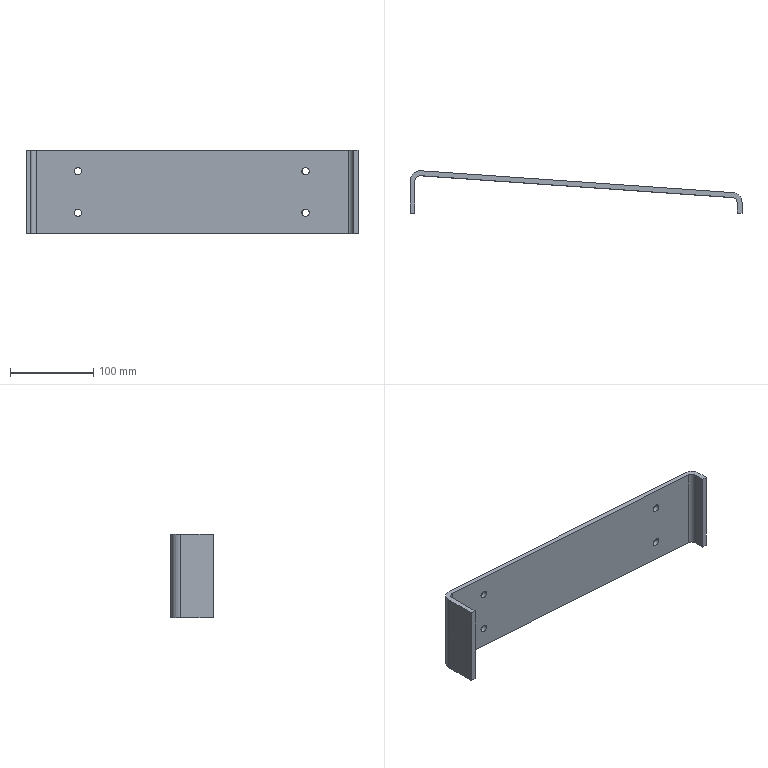Part | SolidWorks | features Fillet 2, Extrusion 1, ICE 1 | 1 solid | 22 faces | box 400 x 51.131 x 100 mm | volume 272755 mm3 | cylinder 12 | plane 10 | commonest cylinder face diameters 9 x8 12 x2 24 x2
STEP:
#1=CARTESIAN_POINT('',(341.245,-29.902,25.));
#2=VERTEX_POINT('',#1);
#3=CARTESIAN_POINT('',(332.267,-29.273,25.));
#4=VERTEX_POINT('',#3);
#5=CARTESIAN_POINT('',(336.756,-29.588,25.));
#6=DIRECTION('',(0.06983,0.9976,0.));
#7=DIRECTION('',(-0.9976,0.06983,0.));
#8=AXIS2_PLACEMENT_3D('',#5,#6,#7);
#9=CIRCLE('',#8,4.5);
#10=EDGE_CURVE('',#2,#4,#9,.T.);
#11=ORIENTED_EDGE('',*,*,#10,.F.);
#12=CARTESIAN_POINT('',(341.664,-23.916,25.));
#13=VERTEX_POINT('',#12);
#14=CARTESIAN_POINT('',(334.681,-123.672,25.));
#15=DIRECTION('',(0.06983,0.9976,0.));
#16=VECTOR('',#15,1000.);
#17=LINE('',#14,#16);
#18=EDGE_CURVE('',#2,#13,#17,.T.);
#19=ORIENTED_EDGE('',*,*,#18,.T.);
#20=CARTESIAN_POINT('',(332.686,-23.288,25.));
#21=VERTEX_POINT('',#20);
#22=CARTESIAN_POINT('',(337.175,-23.602,25.));
#23=DIRECTION('',(0.06983,0.9976,0.));
#24=DIRECTION('',(-0.9976,0.06983,0.));
#25=AXIS2_PLACEMENT_3D('',#22,#23,#24);
#26=CIRCLE('',#25,4.5);
#27=EDGE_CURVE('',#13,#21,#26,.T.);
#28=ORIENTED_EDGE('',*,*,#27,.T.);
#29=CARTESIAN_POINT('',(325.703,-123.044,25.));
#30=DIRECTION('',(0.06983,0.9976,0.));
#31=VECTOR('',#30,1000.);
#32=LINE('',#29,#31);
#33=EDGE_CURVE('',#4,#21,#32,.T.);
#34=ORIENTED_EDGE('',*,*,#33,.F.);
#35=EDGE_LOOP('',(#11,#19,#28,#34));
#36=FACE_OUTER_BOUND('',#35,.T.);
#37=CARTESIAN_POINT('',(330.192,-123.358,25.));
#38=DIRECTION('',(0.06983,0.9976,0.));
#39=DIRECTION('',(-0.9976,0.06983,0.));
#40=AXIS2_PLACEMENT_3D('',#37,#38,#39);
#41=CYLINDRICAL_SURFACE('',#40,4.5);
#42=ADVANCED_FACE('',(#36),#41,.F.);
#43=CARTESIAN_POINT('',(66.916,-10.699,75.));
#44=VERTEX_POINT('',#43);
#45=CARTESIAN_POINT('',(57.938,-10.07,75.));
#46=VERTEX_POINT('',#45);
#47=CARTESIAN_POINT('',(62.427,-10.385,75.));
#48=DIRECTION('',(0.06983,0.9976,0.));
#49=DIRECTION('',(-0.9976,0.06983,0.));
#50=AXIS2_PLACEMENT_3D('',#47,#48,#49);
#51=CIRCLE('',#50,4.5);
#52=EDGE_CURVE('',#44,#46,#51,.T.);
#53=ORIENTED_EDGE('',*,*,#52,.F.);
#54=CARTESIAN_POINT('',(67.335,-4.713,75.));
#55=VERTEX_POINT('',#54);
#56=CARTESIAN_POINT('',(60.352,-104.469,75.));
#57=DIRECTION('',(0.06983,0.9976,0.));
#58=VECTOR('',#57,1000.);
#59=LINE('',#56,#58);
#60=EDGE_CURVE('',#44,#55,#59,.T.);
#61=ORIENTED_EDGE('',*,*,#60,.T.);
#62=CARTESIAN_POINT('',(58.357,-4.085,75.));
#63=VERTEX_POINT('',#62);
#64=CARTESIAN_POINT('',(62.846,-4.399,75.));
#65=DIRECTION('',(0.06983,0.9976,0.));
#66=DIRECTION('',(-0.9976,0.06983,0.));
#67=AXIS2_PLACEMENT_3D('',#64,#65,#66);
#68=CIRCLE('',#67,4.5);
#69=EDGE_CURVE('',#55,#63,#68,.T.);
#70=ORIENTED_EDGE('',*,*,#69,.T.);
#71=CARTESIAN_POINT('',(51.374,-103.841,75.));
#72=DIRECTION('',(0.06983,0.9976,0.));
#73=VECTOR('',#72,1000.);
#74=LINE('',#71,#73);
#75=EDGE_CURVE('',#46,#63,#74,.T.);
#76=ORIENTED_EDGE('',*,*,#75,.F.);
#77=EDGE_LOOP('',(#53,#61,#70,#76));
#78=FACE_OUTER_BOUND('',#77,.T.);
#79=CARTESIAN_POINT('',(55.863,-104.155,75.));
#80=DIRECTION('',(0.06983,0.9976,0.));
#81=DIRECTION('',(-0.9976,0.06983,0.));
#82=AXIS2_PLACEMENT_3D('',#79,#80,#81);
#83=CYLINDRICAL_SURFACE('',#82,4.5);
#84=ADVANCED_FACE('',(#78),#83,.F.);
#85=CARTESIAN_POINT('',(341.245,-29.902,75.));
#86=VERTEX_POINT('',#85);
#87=CARTESIAN_POINT('',(332.267,-29.273,75.));
#88=VERTEX_POINT('',#87);
#89=CARTESIAN_POINT('',(336.756,-29.588,75.));
#90=DIRECTION('',(0.06983,0.9976,0.));
#91=DIRECTION('',(-0.9976,0.06983,0.));
#92=AXIS2_PLACEMENT_3D('',#89,#90,#91);
#93=CIRCLE('',#92,4.5);
#94=EDGE_CURVE('',#86,#88,#93,.T.);
#95=ORIENTED_EDGE('',*,*,#94,.F.);
#96=CARTESIAN_POINT('',(341.664,-23.916,75.));
#97=VERTEX_POINT('',#96);
#98=CARTESIAN_POINT('',(334.681,-123.672,75.));
#99=DIRECTION('',(0.06983,0.9976,0.));
#100=VECTOR('',#99,1000.);
#101=LINE('',#98,#100);
#102=EDGE_CURVE('',#86,#97,#101,.T.);
#103=ORIENTED_EDGE('',*,*,#102,.T.);
#104=CARTESIAN_POINT('',(332.686,-23.288,75.));
#105=VERTEX_POINT('',#104);
#106=CARTESIAN_POINT('',(337.175,-23.602,75.));
#107=DIRECTION('',(0.06983,0.9976,0.));
#108=DIRECTION('',(-0.9976,0.06983,0.));
#109=AXIS2_PLACEMENT_3D('',#106,#107,#108);
#110=CIRCLE('',#109,4.5);
#111=EDGE_CURVE('',#97,#105,#110,.T.);
#112=ORIENTED_EDGE('',*,*,#111,.T.);
#113=CARTESIAN_POINT('',(325.703,-123.044,75.));
#114=DIRECTION('',(0.06983,0.9976,0.));
#115=VECTOR('',#114,1000.);
#116=LINE('',#113,#115);
#117=EDGE_CURVE('',#88,#105,#116,.T.);
#118=ORIENTED_EDGE('',*,*,#117,.F.);
#119=EDGE_LOOP('',(#95,#103,#112,#118));
#120=FACE_OUTER_BOUND('',#119,.T.);
#121=CARTESIAN_POINT('',(330.192,-123.358,75.));
#122=DIRECTION('',(0.06983,0.9976,0.));
#123=DIRECTION('',(-0.9976,0.06983,0.));
#124=AXIS2_PLACEMENT_3D('',#121,#122,#123);
#125=CYLINDRICAL_SURFACE('',#124,4.5);
#126=ADVANCED_FACE('',(#120),#125,.F.);
#127=CARTESIAN_POINT('',(66.916,-10.699,25.));
#128=VERTEX_POINT('',#127);
#129=CARTESIAN_POINT('',(57.938,-10.07,25.));
#130=VERTEX_POINT('',#129);
#131=CARTESIAN_POINT('',(62.427,-10.385,25.));
#132=DIRECTION('',(0.06983,0.9976,0.));
#133=DIRECTION('',(-0.9976,0.06983,0.));
#134=AXIS2_PLACEMENT_3D('',#131,#132,#133);
#135=CIRCLE('',#134,4.5);
#136=EDGE_CURVE('',#128,#130,#135,.T.);
#137=ORIENTED_EDGE('',*,*,#136,.F.);
#138=CARTESIAN_POINT('',(67.335,-4.713,25.));
#139=VERTEX_POINT('',#138);
#140=CARTESIAN_POINT('',(60.352,-104.469,25.));
#141=DIRECTION('',(0.06983,0.9976,0.));
#142=VECTOR('',#141,1000.);
#143=LINE('',#140,#142);
#144=EDGE_CURVE('',#128,#139,#143,.T.);
#145=ORIENTED_EDGE('',*,*,#144,.T.);
#146=CARTESIAN_POINT('',(58.357,-4.085,25.));
#147=VERTEX_POINT('',#146);
#148=CARTESIAN_POINT('',(62.846,-4.399,25.));
#149=DIRECTION('',(0.06983,0.9976,0.));
#150=DIRECTION('',(-0.9976,0.06983,0.));
#151=AXIS2_PLACEMENT_3D('',#148,#149,#150);
#152=CIRCLE('',#151,4.5);
#153=EDGE_CURVE('',#139,#147,#152,.T.);
#154=ORIENTED_EDGE('',*,*,#153,.T.);
#155=CARTESIAN_POINT('',(51.374,-103.841,25.));
#156=DIRECTION('',(0.06983,0.9976,0.));
#157=VECTOR('',#156,1000.);
#158=LINE('',#155,#157);
#159=EDGE_CURVE('',#130,#147,#158,.T.);
#160=ORIENTED_EDGE('',*,*,#159,.F.);
#161=EDGE_LOOP('',(#137,#145,#154,#160));
#162=FACE_OUTER_BOUND('',#161,.T.);
#163=CARTESIAN_POINT('',(55.863,-104.155,25.));
#164=DIRECTION('',(0.06983,0.9976,0.));
#165=DIRECTION('',(-0.9976,0.06983,0.));
#166=AXIS2_PLACEMENT_3D('',#163,#164,#165);
#167=CYLINDRICAL_SURFACE('',#166,4.5);
#168=ADVANCED_FACE('',(#162),#167,.F.);
#169=CARTESIAN_POINT('',(394.,-52.,100.));
#170=VERTEX_POINT('',#169);
#171=CARTESIAN_POINT('',(394.,-39.189,100.));
#172=VERTEX_POINT('',#171);
#173=CARTESIAN_POINT('',(394.,-52.,100.));
#174=DIRECTION('',(0.,1.,0.));
#175=VECTOR('',#174,1000.);
#176=LINE('',#173,#175);
#177=EDGE_CURVE('',#170,#172,#176,.T.);
#178=ORIENTED_EDGE('',*,*,#177,.T.);
#179=CARTESIAN_POINT('',(394.,-39.189,0.));
#180=VERTEX_POINT('',#179);
#181=CARTESIAN_POINT('',(394.,-39.189,100.));
#182=DIRECTION('',(0.,0.,-1.));
#183=VECTOR('',#182,1000.);
#184=LINE('',#181,#183);
#185=EDGE_CURVE('',#172,#180,#184,.T.);
#186=ORIENTED_EDGE('',*,*,#185,.T.);
#187=CARTESIAN_POINT('',(394.,-52.,0.));
#188=VERTEX_POINT('',#187);
#189=CARTESIAN_POINT('',(394.,-52.,0.));
#190=DIRECTION('',(0.,1.,0.));
#191=VECTOR('',#190,1000.);
#192=LINE('',#189,#191);
#193=EDGE_CURVE('',#188,#180,#192,.T.);
#194=ORIENTED_EDGE('',*,*,#193,.F.);
#195=CARTESIAN_POINT('',(394.,-52.,100.));
#196=DIRECTION('',(0.,0.,-1.));
#197=VECTOR('',#196,1000.);
#198=LINE('',#195,#197);
#199=EDGE_CURVE('',#170,#188,#198,.T.);
#200=ORIENTED_EDGE('',*,*,#199,.F.);
#201=EDGE_LOOP('',(#178,#186,#194,#200));
#202=FACE_OUTER_BOUND('',#201,.T.);
#203=CARTESIAN_POINT('',(394.,-52.,100.));
#204=DIRECTION('',(-1.,0.,0.));
#205=DIRECTION('',(0.,0.,1.));
#206=AXIS2_PLACEMENT_3D('',#203,#204,#205);
#207=PLANE('',#206);
#208=ADVANCED_FACE('',(#202),#207,.T.);
#209=CARTESIAN_POINT('',(400.,-52.,0.));
#210=VERTEX_POINT('',#209);
#211=CARTESIAN_POINT('',(394.,-52.,0.));
#212=DIRECTION('',(1.,0.,0.));
#213=VECTOR('',#212,1000.);
#214=LINE('',#211,#213);
#215=EDGE_CURVE('',#188,#210,#214,.T.);
#216=ORIENTED_EDGE('',*,*,#215,.T.);
#217=CARTESIAN_POINT('',(400.,-52.,100.));
#218=VERTEX_POINT('',#217);
#219=CARTESIAN_POINT('',(400.,-52.,100.));
#220=DIRECTION('',(0.,0.,-1.));
#221=VECTOR('',#220,1000.);
#222=LINE('',#219,#221);
#223=EDGE_CURVE('',#218,#210,#222,.T.);
#224=ORIENTED_EDGE('',*,*,#223,.F.);
#225=CARTESIAN_POINT('',(394.,-52.,100.));
#226=DIRECTION('',(1.,0.,0.));
#227=VECTOR('',#226,1000.);
#228=LINE('',#225,#227);
#229=EDGE_CURVE('',#170,#218,#228,.T.);
#230=ORIENTED_EDGE('',*,*,#229,.F.);
#231=ORIENTED_EDGE('',*,*,#199,.T.);
#232=EDGE_LOOP('',(#216,#224,#230,#231));
#233=FACE_OUTER_BOUND('',#232,.T.);
#234=CARTESIAN_POINT('',(394.,-52.,100.));
#235=DIRECTION('',(0.,1.,0.));
#236=DIRECTION('',(0.,0.,1.));
#237=AXIS2_PLACEMENT_3D('',#234,#235,#236);
#238=PLANE('',#237);
#239=ADVANCED_FACE('',(#233),#238,.F.);
#240=CARTESIAN_POINT('',(400.,-39.189,0.));
#241=VERTEX_POINT('',#240);
#242=CARTESIAN_POINT('',(400.,-52.,0.));
#243=DIRECTION('',(0.,1.,0.));
#244=VECTOR('',#243,1000.);
#245=LINE('',#242,#244);
#246=EDGE_CURVE('',#210,#241,#245,.T.);
#247=ORIENTED_EDGE('',*,*,#246,.T.);
#248=CARTESIAN_POINT('',(400.,-39.189,100.));
#249=VERTEX_POINT('',#248);
#250=CARTESIAN_POINT('',(400.,-39.189,100.));
#251=DIRECTION('',(0.,0.,1.));
#252=VECTOR('',#251,1000.);
#253=LINE('',#250,#252);
#254=EDGE_CURVE('',#241,#249,#253,.T.);
#255=ORIENTED_EDGE('',*,*,#254,.T.);
#256=CARTESIAN_POINT('',(400.,-52.,100.));
#257=DIRECTION('',(0.,1.,0.));
#258=VECTOR('',#257,1000.);
#259=LINE('',#256,#258);
#260=EDGE_CURVE('',#218,#249,#259,.T.);
#261=ORIENTED_EDGE('',*,*,#260,.F.);
#262=ORIENTED_EDGE('',*,*,#223,.T.);
#263=EDGE_LOOP('',(#247,#255,#261,#262));
#264=FACE_OUTER_BOUND('',#263,.T.);
#265=CARTESIAN_POINT('',(400.,-52.,100.));
#266=DIRECTION('',(-1.,0.,0.));
#267=DIRECTION('',(0.,0.,1.));
#268=AXIS2_PLACEMENT_3D('',#265,#266,#267);
#269=PLANE('',#268);
#270=ADVANCED_FACE('',(#264),#269,.F.);
#271=CARTESIAN_POINT('',(337.175,-23.602,25.));
#272=DIRECTION('',(0.06983,0.9976,0.));
#273=DIRECTION('',(-0.9976,0.06983,0.));
#274=AXIS2_PLACEMENT_3D('',#271,#272,#273);
#275=CIRCLE('',#274,4.5);
#276=EDGE_CURVE('',#21,#13,#275,.T.);
#277=ORIENTED_EDGE('',*,*,#276,.F.);
#278=ORIENTED_EDGE('',*,*,#27,.F.);
#279=EDGE_LOOP('',(#277,#278));
#280=FACE_BOUND('',#279,.T.);
#281=CARTESIAN_POINT('',(62.846,-4.399,75.));
#282=DIRECTION('',(0.06983,0.9976,0.));
#283=DIRECTION('',(-0.9976,0.06983,0.));
#284=AXIS2_PLACEMENT_3D('',#281,#282,#283);
#285=CIRCLE('',#284,4.5);
#286=EDGE_CURVE('',#63,#55,#285,.T.);
#287=ORIENTED_EDGE('',*,*,#286,.F.);
#288=ORIENTED_EDGE('',*,*,#69,.F.);
#289=EDGE_LOOP('',(#287,#288));
#290=FACE_BOUND('',#289,.T.);
#291=CARTESIAN_POINT('',(337.175,-23.602,75.));
#292=DIRECTION('',(0.06983,0.9976,0.));
#293=DIRECTION('',(-0.9976,0.06983,0.));
#294=AXIS2_PLACEMENT_3D('',#291,#292,#293);
#295=CIRCLE('',#294,4.5);
#296=EDGE_CURVE('',#105,#97,#295,.T.);
#297=ORIENTED_EDGE('',*,*,#296,.F.);
#298=ORIENTED_EDGE('',*,*,#111,.F.);
#299=EDGE_LOOP('',(#297,#298));
#300=FACE_BOUND('',#299,.T.);
#301=CARTESIAN_POINT('',(62.846,-4.399,25.));
#302=DIRECTION('',(0.06983,0.9976,0.));
#303=DIRECTION('',(-0.9976,0.06983,0.));
#304=AXIS2_PLACEMENT_3D('',#301,#302,#303);
#305=CIRCLE('',#304,4.5);
#306=EDGE_CURVE('',#147,#139,#305,.T.);
#307=ORIENTED_EDGE('',*,*,#306,.F.);
#308=ORIENTED_EDGE('',*,*,#153,.F.);
#309=EDGE_LOOP('',(#307,#308));
#310=FACE_BOUND('',#309,.T.);
#311=CARTESIAN_POINT('',(12.838,-0.8987,100.));
#312=VERTEX_POINT('',#311);
#313=CARTESIAN_POINT('',(388.838,-27.219,100.));
#314=VERTEX_POINT('',#313);
#315=CARTESIAN_POINT('',(0.,0.,100.));
#316=DIRECTION('',(0.9976,-0.06983,0.));
#317=VECTOR('',#316,1000.);
#318=LINE('',#315,#317);
#319=EDGE_CURVE('',#312,#314,#318,.T.);
#320=ORIENTED_EDGE('',*,*,#319,.T.);
#321=CARTESIAN_POINT('',(388.838,-27.219,0.));
#322=VERTEX_POINT('',#321);
#323=CARTESIAN_POINT('',(388.838,-27.219,0.));
#324=DIRECTION('',(0.,0.,-1.));
#325=VECTOR('',#324,1000.);
#326=LINE('',#323,#325);
#327=EDGE_CURVE('',#314,#322,#326,.T.);
#328=ORIENTED_EDGE('',*,*,#327,.T.);
#329=CARTESIAN_POINT('',(12.838,-0.8987,0.));
#330=VERTEX_POINT('',#329);
#331=CARTESIAN_POINT('',(0.,0.,0.));
#332=DIRECTION('',(0.9976,-0.06983,0.));
#333=VECTOR('',#332,1000.);
#334=LINE('',#331,#333);
#335=EDGE_CURVE('',#330,#322,#334,.T.);
#336=ORIENTED_EDGE('',*,*,#335,.F.);
#337=CARTESIAN_POINT('',(12.838,-0.8987,100.));
#338=DIRECTION('',(0.,0.,1.));
#339=VECTOR('',#338,1000.);
#340=LINE('',#337,#339);
#341=EDGE_CURVE('',#330,#312,#340,.T.);
#342=ORIENTED_EDGE('',*,*,#341,.T.);
#343=EDGE_LOOP('',(#320,#328,#336,#342));
#344=FACE_OUTER_BOUND('',#343,.T.);
#345=CARTESIAN_POINT('',(0.,0.,100.));
#346=DIRECTION('',(0.06983,0.9976,0.));
#347=DIRECTION('',(-0.9976,0.06983,0.));
#348=AXIS2_PLACEMENT_3D('',#345,#346,#347);
#349=PLANE('',#348);
#350=ADVANCED_FACE('',(#280,#290,#300,#310,#344),#349,.T.);
#351=CARTESIAN_POINT('',(0.,-12.869,100.));
#352=VERTEX_POINT('',#351);
#353=CARTESIAN_POINT('',(0.,-52.,100.));
#354=VERTEX_POINT('',#353);
#355=CARTESIAN_POINT('',(0.,0.,100.));
#356=DIRECTION('',(0.,-1.,0.));
#357=VECTOR('',#356,1000.);
#358=LINE('',#355,#357);
#359=EDGE_CURVE('',#352,#354,#358,.T.);
#360=ORIENTED_EDGE('',*,*,#359,.F.);
#361=CARTESIAN_POINT('',(0.,-12.869,0.));
#362=VERTEX_POINT('',#361);
#363=CARTESIAN_POINT('',(0.,-12.869,0.));
#364=DIRECTION('',(0.,0.,-1.));
#365=VECTOR('',#364,1000.);
#366=LINE('',#363,#365);
#367=EDGE_CURVE('',#352,#362,#366,.T.);
#368=ORIENTED_EDGE('',*,*,#367,.T.);
#369=CARTESIAN_POINT('',(0.,-52.,0.));
#370=VERTEX_POINT('',#369);
#371=CARTESIAN_POINT('',(0.,0.,0.));
#372=DIRECTION('',(0.,-1.,0.));
#373=VECTOR('',#372,1000.);
#374=LINE('',#371,#373);
#375=EDGE_CURVE('',#362,#370,#374,.T.);
#376=ORIENTED_EDGE('',*,*,#375,.T.);
#377=CARTESIAN_POINT('',(0.,-52.,100.));
#378=DIRECTION('',(0.,0.,-1.));
#379=VECTOR('',#378,1000.);
#380=LINE('',#377,#379);
#381=EDGE_CURVE('',#354,#370,#380,.T.);
#382=ORIENTED_EDGE('',*,*,#381,.F.);
#383=EDGE_LOOP('',(#360,#368,#376,#382));
#384=FACE_OUTER_BOUND('',#383,.T.);
#385=CARTESIAN_POINT('',(0.,0.,100.));
#386=DIRECTION('',(1.,0.,0.));
#387=DIRECTION('',(0.,0.,-1.));
#388=AXIS2_PLACEMENT_3D('',#385,#386,#387);
#389=PLANE('',#388);
#390=ADVANCED_FACE('',(#384),#389,.F.);
#391=CARTESIAN_POINT('',(6.,-52.,0.));
#392=VERTEX_POINT('',#391);
#393=CARTESIAN_POINT('',(6.,-52.,0.));
#394=DIRECTION('',(-1.,0.,0.));
#395=VECTOR('',#394,1000.);
#396=LINE('',#393,#395);
#397=EDGE_CURVE('',#392,#370,#396,.T.);
#398=ORIENTED_EDGE('',*,*,#397,.F.);
#399=CARTESIAN_POINT('',(6.,-52.,100.));
#400=VERTEX_POINT('',#399);
#401=CARTESIAN_POINT('',(6.,-52.,100.));
#402=DIRECTION('',(0.,0.,-1.));
#403=VECTOR('',#402,1000.);
#404=LINE('',#401,#403);
#405=EDGE_CURVE('',#400,#392,#404,.T.);
#406=ORIENTED_EDGE('',*,*,#405,.F.);
#407=CARTESIAN_POINT('',(6.,-52.,100.));
#408=DIRECTION('',(-1.,0.,0.));
#409=VECTOR('',#408,1000.);
#410=LINE('',#407,#409);
#411=EDGE_CURVE('',#400,#354,#410,.T.);
#412=ORIENTED_EDGE('',*,*,#411,.T.);
#413=ORIENTED_EDGE('',*,*,#381,.T.);
#414=EDGE_LOOP('',(#398,#406,#412,#413));
#415=FACE_OUTER_BOUND('',#414,.T.);
#416=CARTESIAN_POINT('',(6.,-52.,100.));
#417=DIRECTION('',(0.,-1.,0.));
#418=DIRECTION('',(0.,0.,-1.));
#419=AXIS2_PLACEMENT_3D('',#416,#417,#418);
#420=PLANE('',#419);
#421=ADVANCED_FACE('',(#415),#420,.T.);
#422=CARTESIAN_POINT('',(6.,-12.869,0.));
#423=VERTEX_POINT('',#422);
#424=CARTESIAN_POINT('',(6.,-6.435,0.));
#425=DIRECTION('',(0.,-1.,0.));
#426=VECTOR('',#425,1000.);
#427=LINE('',#424,#426);
#428=EDGE_CURVE('',#423,#392,#427,.T.);
#429=ORIENTED_EDGE('',*,*,#428,.F.);
#430=CARTESIAN_POINT('',(6.,-12.869,100.));
#431=VERTEX_POINT('',#430);
#432=CARTESIAN_POINT('',(6.,-12.869,100.));
#433=DIRECTION('',(0.,0.,1.));
#434=VECTOR('',#433,1000.);
#435=LINE('',#432,#434);
#436=EDGE_CURVE('',#423,#431,#435,.T.);
#437=ORIENTED_EDGE('',*,*,#436,.T.);
#438=CARTESIAN_POINT('',(6.,-6.435,100.));
#439=DIRECTION('',(0.,-1.,0.));
#440=VECTOR('',#439,1000.);
#441=LINE('',#438,#440);
#442=EDGE_CURVE('',#431,#400,#441,.T.);
#443=ORIENTED_EDGE('',*,*,#442,.T.);
#444=ORIENTED_EDGE('',*,*,#405,.T.);
#445=EDGE_LOOP('',(#429,#437,#443,#444));
#446=FACE_OUTER_BOUND('',#445,.T.);
#447=CARTESIAN_POINT('',(6.,-6.435,100.));
#448=DIRECTION('',(1.,0.,0.));
#449=DIRECTION('',(0.,0.,-1.));
#450=AXIS2_PLACEMENT_3D('',#447,#448,#449);
#451=PLANE('',#450);
#452=ADVANCED_FACE('',(#446),#451,.T.);
#453=CARTESIAN_POINT('',(336.756,-29.588,25.));
#454=DIRECTION('',(0.06983,0.9976,0.));
#455=DIRECTION('',(-0.9976,0.06983,0.));
#456=AXIS2_PLACEMENT_3D('',#453,#454,#455);
#457=CIRCLE('',#456,4.5);
#458=EDGE_CURVE('',#4,#2,#457,.T.);
#459=ORIENTED_EDGE('',*,*,#458,.T.);
#460=ORIENTED_EDGE('',*,*,#10,.T.);
#461=EDGE_LOOP('',(#459,#460));
#462=FACE_BOUND('',#461,.T.);
#463=CARTESIAN_POINT('',(62.427,-10.385,75.));
#464=DIRECTION('',(0.06983,0.9976,0.));
#465=DIRECTION('',(-0.9976,0.06983,0.));
#466=AXIS2_PLACEMENT_3D('',#463,#464,#465);
#467=CIRCLE('',#466,4.5);
#468=EDGE_CURVE('',#46,#44,#467,.T.);
#469=ORIENTED_EDGE('',*,*,#468,.T.);
#470=ORIENTED_EDGE('',*,*,#52,.T.);
#471=EDGE_LOOP('',(#469,#470));
#472=FACE_BOUND('',#471,.T.);
#473=CARTESIAN_POINT('',(336.756,-29.588,75.));
#474=DIRECTION('',(0.06983,0.9976,0.));
#475=DIRECTION('',(-0.9976,0.06983,0.));
#476=AXIS2_PLACEMENT_3D('',#473,#474,#475);
#477=CIRCLE('',#476,4.5);
#478=EDGE_CURVE('',#88,#86,#477,.T.);
#479=ORIENTED_EDGE('',*,*,#478,.T.);
#480=ORIENTED_EDGE('',*,*,#94,.T.);
#481=EDGE_LOOP('',(#479,#480));
#482=FACE_BOUND('',#481,.T.);
#483=CARTESIAN_POINT('',(62.427,-10.385,25.));
#484=DIRECTION('',(0.06983,0.9976,0.));
#485=DIRECTION('',(-0.9976,0.06983,0.));
#486=AXIS2_PLACEMENT_3D('',#483,#484,#485);
#487=CIRCLE('',#486,4.5);
#488=EDGE_CURVE('',#130,#128,#487,.T.);
#489=ORIENTED_EDGE('',*,*,#488,.T.);
#490=ORIENTED_EDGE('',*,*,#136,.T.);
#491=EDGE_LOOP('',(#489,#490));
#492=FACE_BOUND('',#491,.T.);
#493=CARTESIAN_POINT('',(12.419,-6.884,0.));
#494=VERTEX_POINT('',#493);
#495=CARTESIAN_POINT('',(388.419,-33.204,0.));
#496=VERTEX_POINT('',#495);
#497=CARTESIAN_POINT('',(6.,-6.435,0.));
#498=DIRECTION('',(0.9976,-0.06983,0.));
#499=VECTOR('',#498,1000.);
#500=LINE('',#497,#499);
#501=EDGE_CURVE('',#494,#496,#500,.T.);
#502=ORIENTED_EDGE('',*,*,#501,.T.);
#503=CARTESIAN_POINT('',(388.419,-33.204,100.));
#504=VERTEX_POINT('',#503);
#505=CARTESIAN_POINT('',(388.419,-33.204,100.));
#506=DIRECTION('',(0.,0.,1.));
#507=VECTOR('',#506,1000.);
#508=LINE('',#505,#507);
#509=EDGE_CURVE('',#496,#504,#508,.T.);
#510=ORIENTED_EDGE('',*,*,#509,.T.);
#511=CARTESIAN_POINT('',(12.419,-6.884,100.));
#512=VERTEX_POINT('',#511);
#513=CARTESIAN_POINT('',(6.,-6.435,100.));
#514=DIRECTION('',(0.9976,-0.06983,0.));
#515=VECTOR('',#514,1000.);
#516=LINE('',#513,#515);
#517=EDGE_CURVE('',#512,#504,#516,.T.);
#518=ORIENTED_EDGE('',*,*,#517,.F.);
#519=CARTESIAN_POINT('',(12.419,-6.884,100.));
#520=DIRECTION('',(0.,0.,-1.));
#521=VECTOR('',#520,1000.);
#522=LINE('',#519,#521);
#523=EDGE_CURVE('',#512,#494,#522,.T.);
#524=ORIENTED_EDGE('',*,*,#523,.T.);
#525=EDGE_LOOP('',(#502,#510,#518,#524));
#526=FACE_OUTER_BOUND('',#525,.T.);
#527=CARTESIAN_POINT('',(6.,-6.435,100.));
#528=DIRECTION('',(0.06983,0.9976,0.));
#529=DIRECTION('',(-0.9976,0.06983,0.));
#530=AXIS2_PLACEMENT_3D('',#527,#528,#529);
#531=PLANE('',#530);
#532=ADVANCED_FACE('',(#462,#472,#482,#492,#526),#531,.F.);
#533=ORIENTED_EDGE('',*,*,#260,.T.);
#534=CARTESIAN_POINT('',(388.,-39.189,100.));
#535=DIRECTION('',(0.,0.,1.));
#536=DIRECTION('',(1.,0.,0.));
#537=AXIS2_PLACEMENT_3D('',#534,#535,#536);
#538=CIRCLE('',#537,12.);
#539=EDGE_CURVE('',#249,#314,#538,.T.);
#540=ORIENTED_EDGE('',*,*,#539,.T.);
#541=ORIENTED_EDGE('',*,*,#319,.F.);
#542=CARTESIAN_POINT('',(12.,-12.869,100.));
#543=DIRECTION('',(0.,0.,1.));
#544=DIRECTION('',(1.,0.,0.));
#545=AXIS2_PLACEMENT_3D('',#542,#543,#544);
#546=CIRCLE('',#545,12.);
#547=EDGE_CURVE('',#312,#352,#546,.T.);
#548=ORIENTED_EDGE('',*,*,#547,.T.);
#549=ORIENTED_EDGE('',*,*,#359,.T.);
#550=ORIENTED_EDGE('',*,*,#411,.F.);
#551=ORIENTED_EDGE('',*,*,#442,.F.);
#552=CARTESIAN_POINT('',(12.,-12.869,100.));
#553=DIRECTION('',(0.,0.,-1.));
#554=DIRECTION('',(1.,0.,0.));
#555=AXIS2_PLACEMENT_3D('',#552,#553,#554);
#556=CIRCLE('',#555,6.);
#557=EDGE_CURVE('',#431,#512,#556,.T.);
#558=ORIENTED_EDGE('',*,*,#557,.T.);
#559=ORIENTED_EDGE('',*,*,#517,.T.);
#560=CARTESIAN_POINT('',(388.,-39.189,100.));
#561=DIRECTION('',(0.,0.,-1.));
#562=DIRECTION('',(1.,0.,0.));
#563=AXIS2_PLACEMENT_3D('',#560,#561,#562);
#564=CIRCLE('',#563,6.);
#565=EDGE_CURVE('',#504,#172,#564,.T.);
#566=ORIENTED_EDGE('',*,*,#565,.T.);
#567=ORIENTED_EDGE('',*,*,#177,.F.);
#568=ORIENTED_EDGE('',*,*,#229,.T.);
#569=EDGE_LOOP('',(#533,#540,#541,#548,#549,#550,#551,#558,#559,#566,#567,#568));
#570=FACE_OUTER_BOUND('',#569,.T.);
#571=CARTESIAN_POINT('',(0.,0.,100.));
#572=DIRECTION('',(0.,0.,1.));
#573=DIRECTION('',(1.,0.,0.));
#574=AXIS2_PLACEMENT_3D('',#571,#572,#573);
#575=PLANE('',#574);
#576=ADVANCED_FACE('',(#570),#575,.T.);
#577=ORIENTED_EDGE('',*,*,#335,.T.);
#578=CARTESIAN_POINT('',(388.,-39.189,0.));
#579=DIRECTION('',(0.,0.,-1.));
#580=DIRECTION('',(1.,0.,0.));
#581=AXIS2_PLACEMENT_3D('',#578,#579,#580);
#582=CIRCLE('',#581,12.);
#583=EDGE_CURVE('',#322,#241,#582,.T.);
#584=ORIENTED_EDGE('',*,*,#583,.T.);
#585=ORIENTED_EDGE('',*,*,#246,.F.);
#586=ORIENTED_EDGE('',*,*,#215,.F.);
#587=ORIENTED_EDGE('',*,*,#193,.T.);
#588=CARTESIAN_POINT('',(388.,-39.189,0.));
#589=DIRECTION('',(0.,0.,1.));
#590=DIRECTION('',(1.,0.,0.));
#591=AXIS2_PLACEMENT_3D('',#588,#589,#590);
#592=CIRCLE('',#591,6.);
#593=EDGE_CURVE('',#180,#496,#592,.T.);
#594=ORIENTED_EDGE('',*,*,#593,.T.);
#595=ORIENTED_EDGE('',*,*,#501,.F.);
#596=CARTESIAN_POINT('',(12.,-12.869,0.));
#597=DIRECTION('',(0.,0.,1.));
#598=DIRECTION('',(1.,0.,0.));
#599=AXIS2_PLACEMENT_3D('',#596,#597,#598);
#600=CIRCLE('',#599,6.);
#601=EDGE_CURVE('',#494,#423,#600,.T.);
#602=ORIENTED_EDGE('',*,*,#601,.T.);
#603=ORIENTED_EDGE('',*,*,#428,.T.);
#604=ORIENTED_EDGE('',*,*,#397,.T.);
#605=ORIENTED_EDGE('',*,*,#375,.F.);
#606=CARTESIAN_POINT('',(12.,-12.869,0.));
#607=DIRECTION('',(0.,0.,-1.));
#608=DIRECTION('',(1.,0.,0.));
#609=AXIS2_PLACEMENT_3D('',#606,#607,#608);
#610=CIRCLE('',#609,12.);
#611=EDGE_CURVE('',#362,#330,#610,.T.);
#612=ORIENTED_EDGE('',*,*,#611,.T.);
#613=EDGE_LOOP('',(#577,#584,#585,#586,#587,#594,#595,#602,#603,#604,#605,#612));
#614=FACE_OUTER_BOUND('',#613,.T.);
#615=CARTESIAN_POINT('',(0.,0.,0.));
#616=DIRECTION('',(0.,0.,1.));
#617=DIRECTION('',(1.,0.,0.));
#618=AXIS2_PLACEMENT_3D('',#615,#616,#617);
#619=PLANE('',#618);
#620=ADVANCED_FACE('',(#614),#619,.F.);
#621=ORIENTED_EDGE('',*,*,#144,.F.);
#622=ORIENTED_EDGE('',*,*,#488,.F.);
#623=ORIENTED_EDGE('',*,*,#159,.T.);
#624=ORIENTED_EDGE('',*,*,#306,.T.);
#625=EDGE_LOOP('',(#621,#622,#623,#624));
#626=FACE_OUTER_BOUND('',#625,.T.);
#627=CARTESIAN_POINT('',(55.863,-104.155,25.));
#628=DIRECTION('',(0.06983,0.9976,0.));
#629=DIRECTION('',(-0.9976,0.06983,0.));
#630=AXIS2_PLACEMENT_3D('',#627,#628,#629);
#631=CYLINDRICAL_SURFACE('',#630,4.5);
#632=ADVANCED_FACE('',(#626),#631,.F.);
#633=ORIENTED_EDGE('',*,*,#102,.F.);
#634=ORIENTED_EDGE('',*,*,#478,.F.);
#635=ORIENTED_EDGE('',*,*,#117,.T.);
#636=ORIENTED_EDGE('',*,*,#296,.T.);
#637=EDGE_LOOP('',(#633,#634,#635,#636));
#638=FACE_OUTER_BOUND('',#637,.T.);
#639=CARTESIAN_POINT('',(330.192,-123.358,75.));
#640=DIRECTION('',(0.06983,0.9976,0.));
#641=DIRECTION('',(-0.9976,0.06983,0.));
#642=AXIS2_PLACEMENT_3D('',#639,#640,#641);
#643=CYLINDRICAL_SURFACE('',#642,4.5);
#644=ADVANCED_FACE('',(#638),#643,.F.);
#645=ORIENTED_EDGE('',*,*,#60,.F.);
#646=ORIENTED_EDGE('',*,*,#468,.F.);
#647=ORIENTED_EDGE('',*,*,#75,.T.);
#648=ORIENTED_EDGE('',*,*,#286,.T.);
#649=EDGE_LOOP('',(#645,#646,#647,#648));
#650=FACE_OUTER_BOUND('',#649,.T.);
#651=CARTESIAN_POINT('',(55.863,-104.155,75.));
#652=DIRECTION('',(0.06983,0.9976,0.));
#653=DIRECTION('',(-0.9976,0.06983,0.));
#654=AXIS2_PLACEMENT_3D('',#651,#652,#653);
#655=CYLINDRICAL_SURFACE('',#654,4.5);
#656=ADVANCED_FACE('',(#650),#655,.F.);
#657=ORIENTED_EDGE('',*,*,#18,.F.);
#658=ORIENTED_EDGE('',*,*,#458,.F.);
#659=ORIENTED_EDGE('',*,*,#33,.T.);
#660=ORIENTED_EDGE('',*,*,#276,.T.);
#661=EDGE_LOOP('',(#657,#658,#659,#660));
#662=FACE_OUTER_BOUND('',#661,.T.);
#663=CARTESIAN_POINT('',(330.192,-123.358,25.));
#664=DIRECTION('',(0.06983,0.9976,0.));
#665=DIRECTION('',(-0.9976,0.06983,0.));
#666=AXIS2_PLACEMENT_3D('',#663,#664,#665);
#667=CYLINDRICAL_SURFACE('',#666,4.5);
#668=ADVANCED_FACE('',(#662),#667,.F.);
#669=ORIENTED_EDGE('',*,*,#539,.F.);
#670=ORIENTED_EDGE('',*,*,#254,.F.);
#671=ORIENTED_EDGE('',*,*,#583,.F.);
#672=ORIENTED_EDGE('',*,*,#327,.F.);
#673=EDGE_LOOP('',(#669,#670,#671,#672));
#674=FACE_OUTER_BOUND('',#673,.T.);
#675=CARTESIAN_POINT('',(388.,-39.189,100.));
#676=DIRECTION('',(0.,0.,1.));
#677=DIRECTION('',(1.,0.,0.));
#678=AXIS2_PLACEMENT_3D('',#675,#676,#677);
#679=CYLINDRICAL_SURFACE('',#678,12.);
#680=ADVANCED_FACE('',(#674),#679,.T.);
#681=ORIENTED_EDGE('',*,*,#547,.F.);
#682=ORIENTED_EDGE('',*,*,#341,.F.);
#683=ORIENTED_EDGE('',*,*,#611,.F.);
#684=ORIENTED_EDGE('',*,*,#367,.F.);
#685=EDGE_LOOP('',(#681,#682,#683,#684));
#686=FACE_OUTER_BOUND('',#685,.T.);
#687=CARTESIAN_POINT('',(12.,-12.869,100.));
#688=DIRECTION('',(0.,0.,1.));
#689=DIRECTION('',(1.,0.,0.));
#690=AXIS2_PLACEMENT_3D('',#687,#688,#689);
#691=CYLINDRICAL_SURFACE('',#690,12.);
#692=ADVANCED_FACE('',(#686),#691,.T.);
#693=ORIENTED_EDGE('',*,*,#565,.F.);
#694=ORIENTED_EDGE('',*,*,#509,.F.);
#695=ORIENTED_EDGE('',*,*,#593,.F.);
#696=ORIENTED_EDGE('',*,*,#185,.F.);
#697=EDGE_LOOP('',(#693,#694,#695,#696));
#698=FACE_OUTER_BOUND('',#697,.T.);
#699=CARTESIAN_POINT('',(388.,-39.189,100.));
#700=DIRECTION('',(0.,0.,-1.));
#701=DIRECTION('',(-1.,0.,0.));
#702=AXIS2_PLACEMENT_3D('',#699,#700,#701);
#703=CYLINDRICAL_SURFACE('',#702,6.);
#704=ADVANCED_FACE('',(#698),#703,.F.);
#705=ORIENTED_EDGE('',*,*,#557,.F.);
#706=ORIENTED_EDGE('',*,*,#436,.F.);
#707=ORIENTED_EDGE('',*,*,#601,.F.);
#708=ORIENTED_EDGE('',*,*,#523,.F.);
#709=EDGE_LOOP('',(#705,#706,#707,#708));
#710=FACE_OUTER_BOUND('',#709,.T.);
#711=CARTESIAN_POINT('',(12.,-12.869,100.));
#712=DIRECTION('',(0.,0.,-1.));
#713=DIRECTION('',(-1.,0.,0.));
#714=AXIS2_PLACEMENT_3D('',#711,#712,#713);
#715=CYLINDRICAL_SURFACE('',#714,6.);
#716=ADVANCED_FACE('',(#710),#715,.F.);
#717=CLOSED_SHELL('',(#42,#84,#126,#168,#208,#239,#270,#350,#390,#421,#452,#532,#576,#620,#632,#644,#656,#668,#680,#692,#704,#716));
#718=MANIFOLD_SOLID_BREP('',#717);
#719=CARTESIAN_POINT('',(0.,0.,0.));
#720=DIRECTION('',(0.,0.,1.));
#721=DIRECTION('',(1.,0.,0.));
#722=AXIS2_PLACEMENT_3D('',#719,#720,#721);
#723=(LENGTH_UNIT()NAMED_UNIT(*)SI_UNIT(.MILLI.,.METRE.));
#724=UNCERTAINTY_MEASURE_WITH_UNIT(LENGTH_MEASURE(0.00001),#723,'','');
#725=(NAMED_UNIT(*)PLANE_ANGLE_UNIT()SI_UNIT($,.RADIAN.));
#726=(NAMED_UNIT(*)SI_UNIT($,.STERADIAN.)SOLID_ANGLE_UNIT());
#727=(GEOMETRIC_REPRESENTATION_CONTEXT(3)GLOBAL_UNCERTAINTY_ASSIGNED_CONTEXT((#724))GLOBAL_UNIT_ASSIGNED_CONTEXT((#723,#725,#726))REPRESENTATION_CONTEXT('',''));
#728=ADVANCED_BREP_SHAPE_REPRESENTATION('',(#718,#722),#727);